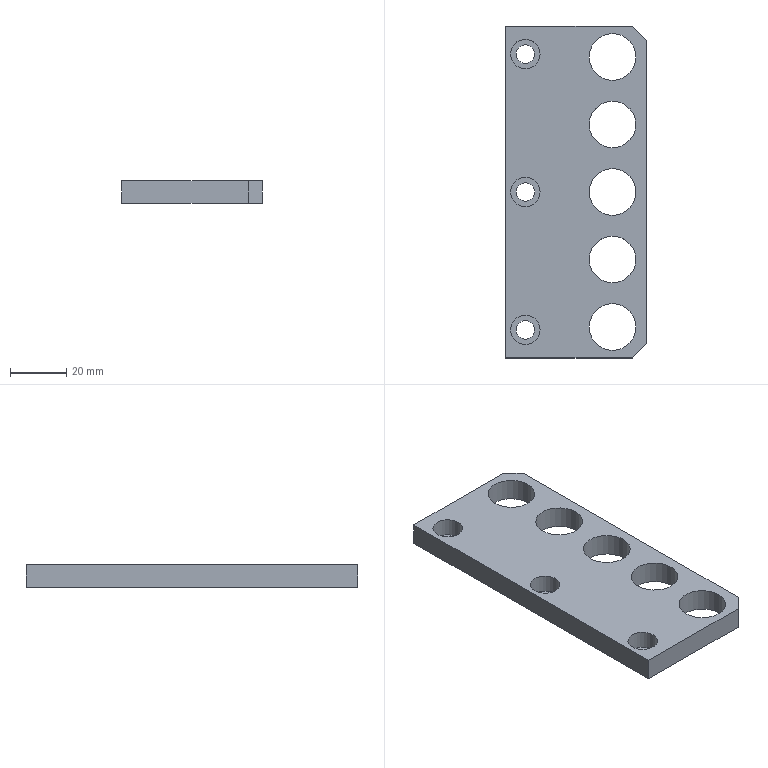NC program | NX | posted with a generic post | part box 50 x 118 x 8 mm
Lines 1 to 54 of 2555:
N10 G17 G21 G94 G90
(PLANAR_MILL , TOOL : D63R0.8)
N12 T01 M6
N14 G54
N16 G17 G0 G90 X96. Y0. S2500 M3
N18 G43 Z30. H1
N20 Z2.
N22 G94 G1 Z0. F800.
N24 X62.5
N26 X-62.5
N28 X-96.
N30 Z2.
N32 G0 Z30.
N34 M5
(DRILLING , TOOL : D6点钻)
N36 T02 M6
N38 G54
N40 G17 G0 G90 X-48. Y13. S2000 M3
N42 G43 Z30. H2
N44 G94 G81 G98 Z-1.5 F150. R3.
N46 X-24.
N48 X0.
N50 X24.
N52 X48.
N54 X49. Y-18.
N56 X0.
N58 X-49.
N60 G80
N62 G0 X-49. Y-18. Z30.
N64 M5
(DRILLING_COPY , TOOL : Z6.5)
N66 T03 M6
N68 G54
N70 G17 G0 G90 X-48. Y13. S2000 M3
N72 G43 Z30. H3
N74 G94 G81 G98 Z-12. F150. R3.
N76 X-24.
N78 X0.
N80 X24.
N82 X48.
N84 X49. Y-18.
N86 X0.
N88 X-49.
N90 G80
N92 G0 X-49. Y-18. Z30.
N94 M5